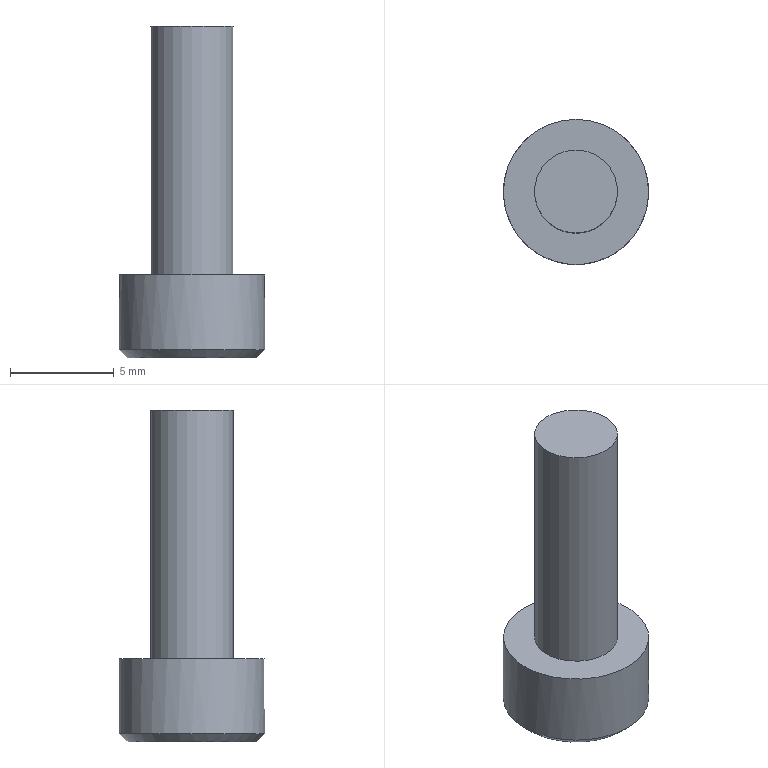Part | NX | features 5003_334_CB4-12 2 | 1 solid | 19 faces | box 7 x 7 x 16 mm | volume 285.33 mm3 | plane 15 | cylinder 2 | cone 2 | commonest cylinder face diameters 4 x1 7 x1
STEP:
#1=CARTESIAN_POINT('',(216.825,63.3,-140.18));
#2=VERTEX_POINT('',#1);
#3=CARTESIAN_POINT('',(216.825,66.4,-140.18));
#4=DIRECTION('',(0.,0.,1.));
#5=DIRECTION('',(0.,-1.,0.));
#6=AXIS2_PLACEMENT_3D('',#3,#4,#5);
#7=CIRCLE('',#6,3.1);
#8=EDGE_CURVE('',#2,#2,#7,.F.);
#9=ORIENTED_EDGE('',*,*,#8,.T.);
#10=EDGE_LOOP('',(#9));
#11=FACE_BOUND('',#10,.T.);
#12=CARTESIAN_POINT('',(215.093,66.4,-140.18));
#13=VERTEX_POINT('',#12);
#14=CARTESIAN_POINT('',(215.959,67.9,-140.18));
#15=VERTEX_POINT('',#14);
#16=CARTESIAN_POINT('',(215.093,66.4,-140.18));
#17=DIRECTION('',(0.5,0.866,0.));
#18=VECTOR('',#17,1000.);
#19=LINE('',#16,#18);
#20=EDGE_CURVE('',#13,#15,#19,.T.);
#21=ORIENTED_EDGE('',*,*,#20,.F.);
#22=CARTESIAN_POINT('',(215.959,64.9,-140.18));
#23=VERTEX_POINT('',#22);
#24=CARTESIAN_POINT('',(215.959,64.9,-140.18));
#25=DIRECTION('',(-0.5,0.866,0.));
#26=VECTOR('',#25,1000.);
#27=LINE('',#24,#26);
#28=EDGE_CURVE('',#23,#13,#27,.T.);
#29=ORIENTED_EDGE('',*,*,#28,.F.);
#30=CARTESIAN_POINT('',(217.691,64.9,-140.18));
#31=VERTEX_POINT('',#30);
#32=CARTESIAN_POINT('',(217.691,64.9,-140.18));
#33=DIRECTION('',(-1.,0.,0.));
#34=VECTOR('',#33,1000.);
#35=LINE('',#32,#34);
#36=EDGE_CURVE('',#31,#23,#35,.T.);
#37=ORIENTED_EDGE('',*,*,#36,.F.);
#38=CARTESIAN_POINT('',(218.557,66.4,-140.18));
#39=VERTEX_POINT('',#38);
#40=CARTESIAN_POINT('',(218.557,66.4,-140.18));
#41=DIRECTION('',(-0.5,-0.866,0.));
#42=VECTOR('',#41,1000.);
#43=LINE('',#40,#42);
#44=EDGE_CURVE('',#39,#31,#43,.T.);
#45=ORIENTED_EDGE('',*,*,#44,.F.);
#46=CARTESIAN_POINT('',(217.691,67.9,-140.18));
#47=VERTEX_POINT('',#46);
#48=CARTESIAN_POINT('',(217.691,67.9,-140.18));
#49=DIRECTION('',(0.5,-0.866,0.));
#50=VECTOR('',#49,1000.);
#51=LINE('',#48,#50);
#52=EDGE_CURVE('',#47,#39,#51,.T.);
#53=ORIENTED_EDGE('',*,*,#52,.F.);
#54=CARTESIAN_POINT('',(215.959,67.9,-140.18));
#55=DIRECTION('',(1.,0.,0.));
#56=VECTOR('',#55,1000.);
#57=LINE('',#54,#56);
#58=EDGE_CURVE('',#15,#47,#57,.T.);
#59=ORIENTED_EDGE('',*,*,#58,.F.);
#60=EDGE_LOOP('',(#21,#29,#37,#45,#53,#59));
#61=FACE_BOUND('',#60,.T.);
#62=CARTESIAN_POINT('',(220.325,66.4,-140.18));
#63=DIRECTION('',(0.,0.,1.));
#64=DIRECTION('',(0.,-1.,0.));
#65=AXIS2_PLACEMENT_3D('',#62,#63,#64);
#66=PLANE('',#65);
#67=ADVANCED_FACE('',(#11,#61),#66,.F.);
#68=CARTESIAN_POINT('',(216.825,68.4,-124.18));
#69=VERTEX_POINT('',#68);
#70=CARTESIAN_POINT('',(216.825,66.4,-124.18));
#71=DIRECTION('',(0.,0.,-1.));
#72=DIRECTION('',(0.,1.,0.));
#73=AXIS2_PLACEMENT_3D('',#70,#71,#72);
#74=CIRCLE('',#73,2.);
#75=EDGE_CURVE('',#69,#69,#74,.T.);
#76=ORIENTED_EDGE('',*,*,#75,.F.);
#77=EDGE_LOOP('',(#76));
#78=FACE_BOUND('',#77,.T.);
#79=CARTESIAN_POINT('',(216.825,66.4,-124.18));
#80=DIRECTION('',(0.,0.,-1.));
#81=DIRECTION('',(0.,1.,0.));
#82=AXIS2_PLACEMENT_3D('',#79,#80,#81);
#83=PLANE('',#82);
#84=ADVANCED_FACE('',(#78),#83,.F.);
#85=CARTESIAN_POINT('',(216.825,68.4,-136.18));
#86=VERTEX_POINT('',#85);
#87=CARTESIAN_POINT('',(216.825,66.4,-136.18));
#88=DIRECTION('',(0.,0.,-1.));
#89=DIRECTION('',(0.,1.,0.));
#90=AXIS2_PLACEMENT_3D('',#87,#88,#89);
#91=CIRCLE('',#90,2.);
#92=EDGE_CURVE('',#86,#86,#91,.T.);
#93=ORIENTED_EDGE('',*,*,#92,.F.);
#94=EDGE_LOOP('',(#93));
#95=FACE_BOUND('',#94,.T.);
#96=ORIENTED_EDGE('',*,*,#75,.T.);
#97=EDGE_LOOP('',(#96));
#98=FACE_BOUND('',#97,.T.);
#99=CARTESIAN_POINT('',(216.825,66.4,-140.18));
#100=DIRECTION('',(0.,0.,-1.));
#101=DIRECTION('',(0.,1.,0.));
#102=AXIS2_PLACEMENT_3D('',#99,#100,#101);
#103=CYLINDRICAL_SURFACE('',#102,2.);
#104=ADVANCED_FACE('',(#95,#98),#103,.T.);
#105=CARTESIAN_POINT('',(216.825,69.9,-136.18));
#106=VERTEX_POINT('',#105);
#107=CARTESIAN_POINT('',(216.825,66.4,-136.18));
#108=DIRECTION('',(0.,0.,-1.));
#109=DIRECTION('',(0.,1.,0.));
#110=AXIS2_PLACEMENT_3D('',#107,#108,#109);
#111=CIRCLE('',#110,3.5);
#112=EDGE_CURVE('',#106,#106,#111,.T.);
#113=ORIENTED_EDGE('',*,*,#112,.F.);
#114=EDGE_LOOP('',(#113));
#115=FACE_BOUND('',#114,.T.);
#116=ORIENTED_EDGE('',*,*,#92,.T.);
#117=EDGE_LOOP('',(#116));
#118=FACE_BOUND('',#117,.T.);
#119=CARTESIAN_POINT('',(218.825,66.4,-136.18));
#120=DIRECTION('',(0.,0.,-1.));
#121=DIRECTION('',(0.,1.,0.));
#122=AXIS2_PLACEMENT_3D('',#119,#120,#121);
#123=PLANE('',#122);
#124=ADVANCED_FACE('',(#115,#118),#123,.F.);
#125=CARTESIAN_POINT('',(216.825,62.9,-139.78));
#126=VERTEX_POINT('',#125);
#127=CARTESIAN_POINT('',(216.825,66.4,-139.78));
#128=DIRECTION('',(0.,0.,1.));
#129=DIRECTION('',(0.,-1.,0.));
#130=AXIS2_PLACEMENT_3D('',#127,#128,#129);
#131=CIRCLE('',#130,3.5);
#132=EDGE_CURVE('',#126,#126,#131,.T.);
#133=ORIENTED_EDGE('',*,*,#132,.T.);
#134=EDGE_LOOP('',(#133));
#135=FACE_BOUND('',#134,.T.);
#136=ORIENTED_EDGE('',*,*,#112,.T.);
#137=EDGE_LOOP('',(#136));
#138=FACE_BOUND('',#137,.T.);
#139=CARTESIAN_POINT('',(216.825,66.4,-140.18));
#140=DIRECTION('',(0.,0.,-1.));
#141=DIRECTION('',(0.,1.,0.));
#142=AXIS2_PLACEMENT_3D('',#139,#140,#141);
#143=CYLINDRICAL_SURFACE('',#142,3.5);
#144=ADVANCED_FACE('',(#135,#138),#143,.T.);
#145=ORIENTED_EDGE('',*,*,#132,.F.);
#146=EDGE_LOOP('',(#145));
#147=FACE_BOUND('',#146,.T.);
#148=ORIENTED_EDGE('',*,*,#8,.F.);
#149=EDGE_LOOP('',(#148));
#150=FACE_BOUND('',#149,.T.);
#151=CARTESIAN_POINT('',(216.825,66.4,-140.18));
#152=DIRECTION('',(0.,0.,1.));
#153=DIRECTION('',(0.,-1.,0.));
#154=AXIS2_PLACEMENT_3D('',#151,#152,#153);
#155=CONICAL_SURFACE('',#154,3.1,0.7854);
#156=ADVANCED_FACE('',(#147,#150),#155,.T.);
#157=CARTESIAN_POINT('',(215.959,64.9,-138.18));
#158=VERTEX_POINT('',#157);
#159=CARTESIAN_POINT('',(215.526,65.65,-138.18));
#160=VERTEX_POINT('',#159);
#161=CARTESIAN_POINT('',(215.959,64.9,-138.18));
#162=DIRECTION('',(-0.5,0.866,0.));
#163=VECTOR('',#162,1000.);
#164=LINE('',#161,#163);
#165=EDGE_CURVE('',#158,#160,#164,.T.);
#166=ORIENTED_EDGE('',*,*,#165,.F.);
#167=CARTESIAN_POINT('',(215.959,64.9,-138.18));
#168=DIRECTION('',(0.,0.,-1.));
#169=VECTOR('',#168,1000.);
#170=LINE('',#167,#169);
#171=EDGE_CURVE('',#158,#23,#170,.T.);
#172=ORIENTED_EDGE('',*,*,#171,.T.);
#173=ORIENTED_EDGE('',*,*,#28,.T.);
#174=CARTESIAN_POINT('',(215.093,66.4,-138.18));
#175=VERTEX_POINT('',#174);
#176=CARTESIAN_POINT('',(215.093,66.4,-138.18));
#177=DIRECTION('',(0.,0.,-1.));
#178=VECTOR('',#177,1000.);
#179=LINE('',#176,#178);
#180=EDGE_CURVE('',#175,#13,#179,.T.);
#181=ORIENTED_EDGE('',*,*,#180,.F.);
#182=CARTESIAN_POINT('',(215.959,64.9,-138.18));
#183=DIRECTION('',(-0.5,0.866,0.));
#184=VECTOR('',#183,1000.);
#185=LINE('',#182,#184);
#186=EDGE_CURVE('',#160,#175,#185,.T.);
#187=ORIENTED_EDGE('',*,*,#186,.F.);
#188=EDGE_LOOP('',(#166,#172,#173,#181,#187));
#189=FACE_BOUND('',#188,.T.);
#190=CARTESIAN_POINT('',(215.959,64.9,-138.18));
#191=DIRECTION('',(-0.866,-0.5,0.));
#192=DIRECTION('',(0.5,-0.866,0.));
#193=AXIS2_PLACEMENT_3D('',#190,#191,#192);
#194=PLANE('',#193);
#195=ADVANCED_FACE('',(#189),#194,.F.);
#196=CARTESIAN_POINT('',(217.691,64.9,-138.18));
#197=VERTEX_POINT('',#196);
#198=CARTESIAN_POINT('',(216.825,64.9,-138.18));
#199=VERTEX_POINT('',#198);
#200=CARTESIAN_POINT('',(217.691,64.9,-138.18));
#201=DIRECTION('',(-1.,0.,0.));
#202=VECTOR('',#201,1000.);
#203=LINE('',#200,#202);
#204=EDGE_CURVE('',#197,#199,#203,.T.);
#205=ORIENTED_EDGE('',*,*,#204,.F.);
#206=CARTESIAN_POINT('',(217.691,64.9,-138.18));
#207=DIRECTION('',(0.,0.,-1.));
#208=VECTOR('',#207,1000.);
#209=LINE('',#206,#208);
#210=EDGE_CURVE('',#197,#31,#209,.T.);
#211=ORIENTED_EDGE('',*,*,#210,.T.);
#212=ORIENTED_EDGE('',*,*,#36,.T.);
#213=ORIENTED_EDGE('',*,*,#171,.F.);
#214=CARTESIAN_POINT('',(217.691,64.9,-138.18));
#215=DIRECTION('',(-1.,0.,0.));
#216=VECTOR('',#215,1000.);
#217=LINE('',#214,#216);
#218=EDGE_CURVE('',#199,#158,#217,.T.);
#219=ORIENTED_EDGE('',*,*,#218,.F.);
#220=EDGE_LOOP('',(#205,#211,#212,#213,#219));
#221=FACE_BOUND('',#220,.T.);
#222=CARTESIAN_POINT('',(217.691,64.9,-138.18));
#223=DIRECTION('',(0.,-1.,0.));
#224=DIRECTION('',(0.,0.,-1.));
#225=AXIS2_PLACEMENT_3D('',#222,#223,#224);
#226=PLANE('',#225);
#227=ADVANCED_FACE('',(#221),#226,.F.);
#228=CARTESIAN_POINT('',(218.557,66.4,-138.18));
#229=VERTEX_POINT('',#228);
#230=CARTESIAN_POINT('',(218.124,65.65,-138.18));
#231=VERTEX_POINT('',#230);
#232=CARTESIAN_POINT('',(218.557,66.4,-138.18));
#233=DIRECTION('',(-0.5,-0.866,0.));
#234=VECTOR('',#233,1000.);
#235=LINE('',#232,#234);
#236=EDGE_CURVE('',#229,#231,#235,.T.);
#237=ORIENTED_EDGE('',*,*,#236,.F.);
#238=CARTESIAN_POINT('',(218.557,66.4,-138.18));
#239=DIRECTION('',(0.,0.,-1.));
#240=VECTOR('',#239,1000.);
#241=LINE('',#238,#240);
#242=EDGE_CURVE('',#229,#39,#241,.T.);
#243=ORIENTED_EDGE('',*,*,#242,.T.);
#244=ORIENTED_EDGE('',*,*,#44,.T.);
#245=ORIENTED_EDGE('',*,*,#210,.F.);
#246=CARTESIAN_POINT('',(218.557,66.4,-138.18));
#247=DIRECTION('',(-0.5,-0.866,0.));
#248=VECTOR('',#247,1000.);
#249=LINE('',#246,#248);
#250=EDGE_CURVE('',#231,#197,#249,.T.);
#251=ORIENTED_EDGE('',*,*,#250,.F.);
#252=EDGE_LOOP('',(#237,#243,#244,#245,#251));
#253=FACE_BOUND('',#252,.T.);
#254=CARTESIAN_POINT('',(218.557,66.4,-138.18));
#255=DIRECTION('',(0.866,-0.5,0.));
#256=DIRECTION('',(0.5,0.866,0.));
#257=AXIS2_PLACEMENT_3D('',#254,#255,#256);
#258=PLANE('',#257);
#259=ADVANCED_FACE('',(#253),#258,.F.);
#260=CARTESIAN_POINT('',(217.691,67.9,-138.18));
#261=VERTEX_POINT('',#260);
#262=CARTESIAN_POINT('',(218.124,67.15,-138.18));
#263=VERTEX_POINT('',#262);
#264=CARTESIAN_POINT('',(217.691,67.9,-138.18));
#265=DIRECTION('',(0.5,-0.866,0.));
#266=VECTOR('',#265,1000.);
#267=LINE('',#264,#266);
#268=EDGE_CURVE('',#261,#263,#267,.T.);
#269=ORIENTED_EDGE('',*,*,#268,.F.);
#270=CARTESIAN_POINT('',(217.691,67.9,-138.18));
#271=DIRECTION('',(0.,0.,-1.));
#272=VECTOR('',#271,1000.);
#273=LINE('',#270,#272);
#274=EDGE_CURVE('',#261,#47,#273,.T.);
#275=ORIENTED_EDGE('',*,*,#274,.T.);
#276=ORIENTED_EDGE('',*,*,#52,.T.);
#277=ORIENTED_EDGE('',*,*,#242,.F.);
#278=CARTESIAN_POINT('',(217.691,67.9,-138.18));
#279=DIRECTION('',(0.5,-0.866,0.));
#280=VECTOR('',#279,1000.);
#281=LINE('',#278,#280);
#282=EDGE_CURVE('',#263,#229,#281,.T.);
#283=ORIENTED_EDGE('',*,*,#282,.F.);
#284=EDGE_LOOP('',(#269,#275,#276,#277,#283));
#285=FACE_BOUND('',#284,.T.);
#286=CARTESIAN_POINT('',(217.691,67.9,-138.18));
#287=DIRECTION('',(0.866,0.5,0.));
#288=DIRECTION('',(-0.5,0.866,0.));
#289=AXIS2_PLACEMENT_3D('',#286,#287,#288);
#290=PLANE('',#289);
#291=ADVANCED_FACE('',(#285),#290,.F.);
#292=CARTESIAN_POINT('',(215.959,67.9,-138.18));
#293=VERTEX_POINT('',#292);
#294=CARTESIAN_POINT('',(216.825,67.9,-138.18));
#295=VERTEX_POINT('',#294);
#296=CARTESIAN_POINT('',(215.959,67.9,-138.18));
#297=DIRECTION('',(1.,0.,0.));
#298=VECTOR('',#297,1000.);
#299=LINE('',#296,#298);
#300=EDGE_CURVE('',#293,#295,#299,.T.);
#301=ORIENTED_EDGE('',*,*,#300,.F.);
#302=CARTESIAN_POINT('',(215.959,67.9,-138.18));
#303=DIRECTION('',(0.,0.,-1.));
#304=VECTOR('',#303,1000.);
#305=LINE('',#302,#304);
#306=EDGE_CURVE('',#293,#15,#305,.T.);
#307=ORIENTED_EDGE('',*,*,#306,.T.);
#308=ORIENTED_EDGE('',*,*,#58,.T.);
#309=ORIENTED_EDGE('',*,*,#274,.F.);
#310=CARTESIAN_POINT('',(215.959,67.9,-138.18));
#311=DIRECTION('',(1.,0.,0.));
#312=VECTOR('',#311,1000.);
#313=LINE('',#310,#312);
#314=EDGE_CURVE('',#295,#261,#313,.T.);
#315=ORIENTED_EDGE('',*,*,#314,.F.);
#316=EDGE_LOOP('',(#301,#307,#308,#309,#315));
#317=FACE_BOUND('',#316,.T.);
#318=CARTESIAN_POINT('',(215.959,67.9,-138.18));
#319=DIRECTION('',(0.,1.,0.));
#320=DIRECTION('',(0.,0.,1.));
#321=AXIS2_PLACEMENT_3D('',#318,#319,#320);
#322=PLANE('',#321);
#323=ADVANCED_FACE('',(#317),#322,.F.);
#324=CARTESIAN_POINT('',(215.526,67.15,-138.18));
#325=VERTEX_POINT('',#324);
#326=CARTESIAN_POINT('',(215.093,66.4,-138.18));
#327=DIRECTION('',(0.5,0.866,0.));
#328=VECTOR('',#327,1000.);
#329=LINE('',#326,#328);
#330=EDGE_CURVE('',#175,#325,#329,.T.);
#331=ORIENTED_EDGE('',*,*,#330,.F.);
#332=ORIENTED_EDGE('',*,*,#180,.T.);
#333=ORIENTED_EDGE('',*,*,#20,.T.);
#334=ORIENTED_EDGE('',*,*,#306,.F.);
#335=CARTESIAN_POINT('',(215.093,66.4,-138.18));
#336=DIRECTION('',(0.5,0.866,0.));
#337=VECTOR('',#336,1000.);
#338=LINE('',#335,#337);
#339=EDGE_CURVE('',#325,#293,#338,.T.);
#340=ORIENTED_EDGE('',*,*,#339,.F.);
#341=EDGE_LOOP('',(#331,#332,#333,#334,#340));
#342=FACE_BOUND('',#341,.T.);
#343=CARTESIAN_POINT('',(215.093,66.4,-138.18));
#344=DIRECTION('',(-0.866,0.5,0.));
#345=DIRECTION('',(-0.5,-0.866,0.));
#346=AXIS2_PLACEMENT_3D('',#343,#344,#345);
#347=PLANE('',#346);
#348=ADVANCED_FACE('',(#342),#347,.F.);
#349=ORIENTED_EDGE('',*,*,#314,.T.);
#350=ORIENTED_EDGE('',*,*,#268,.T.);
#351=CARTESIAN_POINT('',(216.825,66.4,-138.18));
#352=DIRECTION('',(0.,0.,-1.));
#353=DIRECTION('',(-1.,0.,0.));
#354=AXIS2_PLACEMENT_3D('',#351,#352,#353);
#355=CIRCLE('',#354,1.5);
#356=EDGE_CURVE('',#295,#263,#355,.T.);
#357=ORIENTED_EDGE('',*,*,#356,.F.);
#358=EDGE_LOOP('',(#349,#350,#357));
#359=FACE_BOUND('',#358,.T.);
#360=CARTESIAN_POINT('',(216.825,66.4,-138.18));
#361=DIRECTION('',(0.,0.,-1.));
#362=DIRECTION('',(0.,1.,0.));
#363=AXIS2_PLACEMENT_3D('',#360,#361,#362);
#364=PLANE('',#363);
#365=ADVANCED_FACE('',(#359),#364,.T.);
#366=ORIENTED_EDGE('',*,*,#282,.T.);
#367=ORIENTED_EDGE('',*,*,#236,.T.);
#368=CARTESIAN_POINT('',(216.825,66.4,-138.18));
#369=DIRECTION('',(0.,0.,-1.));
#370=DIRECTION('',(-1.,0.,0.));
#371=AXIS2_PLACEMENT_3D('',#368,#369,#370);
#372=CIRCLE('',#371,1.5);
#373=EDGE_CURVE('',#263,#231,#372,.T.);
#374=ORIENTED_EDGE('',*,*,#373,.F.);
#375=EDGE_LOOP('',(#366,#367,#374));
#376=FACE_BOUND('',#375,.T.);
#377=CARTESIAN_POINT('',(216.825,66.4,-138.18));
#378=DIRECTION('',(0.,0.,-1.));
#379=DIRECTION('',(0.,1.,0.));
#380=AXIS2_PLACEMENT_3D('',#377,#378,#379);
#381=PLANE('',#380);
#382=ADVANCED_FACE('',(#376),#381,.T.);
#383=ORIENTED_EDGE('',*,*,#250,.T.);
#384=ORIENTED_EDGE('',*,*,#204,.T.);
#385=CARTESIAN_POINT('',(216.825,66.4,-138.18));
#386=DIRECTION('',(0.,0.,-1.));
#387=DIRECTION('',(-1.,0.,0.));
#388=AXIS2_PLACEMENT_3D('',#385,#386,#387);
#389=CIRCLE('',#388,1.5);
#390=EDGE_CURVE('',#231,#199,#389,.T.);
#391=ORIENTED_EDGE('',*,*,#390,.F.);
#392=EDGE_LOOP('',(#383,#384,#391));
#393=FACE_BOUND('',#392,.T.);
#394=CARTESIAN_POINT('',(216.825,66.4,-138.18));
#395=DIRECTION('',(0.,0.,-1.));
#396=DIRECTION('',(0.,1.,0.));
#397=AXIS2_PLACEMENT_3D('',#394,#395,#396);
#398=PLANE('',#397);
#399=ADVANCED_FACE('',(#393),#398,.T.);
#400=ORIENTED_EDGE('',*,*,#218,.T.);
#401=ORIENTED_EDGE('',*,*,#165,.T.);
#402=CARTESIAN_POINT('',(216.825,66.4,-138.18));
#403=DIRECTION('',(0.,0.,-1.));
#404=DIRECTION('',(-1.,0.,0.));
#405=AXIS2_PLACEMENT_3D('',#402,#403,#404);
#406=CIRCLE('',#405,1.5);
#407=EDGE_CURVE('',#199,#160,#406,.T.);
#408=ORIENTED_EDGE('',*,*,#407,.F.);
#409=EDGE_LOOP('',(#400,#401,#408));
#410=FACE_BOUND('',#409,.T.);
#411=CARTESIAN_POINT('',(216.825,66.4,-138.18));
#412=DIRECTION('',(0.,0.,-1.));
#413=DIRECTION('',(0.,1.,0.));
#414=AXIS2_PLACEMENT_3D('',#411,#412,#413);
#415=PLANE('',#414);
#416=ADVANCED_FACE('',(#410),#415,.T.);
#417=ORIENTED_EDGE('',*,*,#186,.T.);
#418=ORIENTED_EDGE('',*,*,#330,.T.);
#419=CARTESIAN_POINT('',(216.825,66.4,-138.18));
#420=DIRECTION('',(0.,0.,-1.));
#421=DIRECTION('',(-1.,0.,0.));
#422=AXIS2_PLACEMENT_3D('',#419,#420,#421);
#423=CIRCLE('',#422,1.5);
#424=EDGE_CURVE('',#160,#325,#423,.T.);
#425=ORIENTED_EDGE('',*,*,#424,.F.);
#426=EDGE_LOOP('',(#417,#418,#425));
#427=FACE_BOUND('',#426,.T.);
#428=CARTESIAN_POINT('',(216.825,66.4,-138.18));
#429=DIRECTION('',(0.,0.,-1.));
#430=DIRECTION('',(0.,1.,0.));
#431=AXIS2_PLACEMENT_3D('',#428,#429,#430);
#432=PLANE('',#431);
#433=ADVANCED_FACE('',(#427),#432,.T.);
#434=ORIENTED_EDGE('',*,*,#339,.T.);
#435=ORIENTED_EDGE('',*,*,#300,.T.);
#436=CARTESIAN_POINT('',(216.825,66.4,-138.18));
#437=DIRECTION('',(0.,0.,-1.));
#438=DIRECTION('',(-1.,0.,0.));
#439=AXIS2_PLACEMENT_3D('',#436,#437,#438);
#440=CIRCLE('',#439,1.5);
#441=EDGE_CURVE('',#325,#295,#440,.T.);
#442=ORIENTED_EDGE('',*,*,#441,.F.);
#443=EDGE_LOOP('',(#434,#435,#442));
#444=FACE_BOUND('',#443,.T.);
#445=CARTESIAN_POINT('',(216.825,66.4,-138.18));
#446=DIRECTION('',(0.,0.,-1.));
#447=DIRECTION('',(0.,1.,0.));
#448=AXIS2_PLACEMENT_3D('',#445,#446,#447);
#449=PLANE('',#448);
#450=ADVANCED_FACE('',(#444),#449,.T.);
#451=ORIENTED_EDGE('',*,*,#441,.T.);
#452=ORIENTED_EDGE('',*,*,#356,.T.);
#453=ORIENTED_EDGE('',*,*,#373,.T.);
#454=ORIENTED_EDGE('',*,*,#390,.T.);
#455=ORIENTED_EDGE('',*,*,#407,.T.);
#456=ORIENTED_EDGE('',*,*,#424,.T.);
#457=EDGE_LOOP('',(#451,#452,#453,#454,#455,#456));
#458=FACE_BOUND('',#457,.T.);
#459=CARTESIAN_POINT('',(216.825,66.4,-137.279));
#460=VERTEX_POINT('',#459);
#461=VERTEX_LOOP('',#460);
#462=FACE_BOUND('',#461,.T.);
#463=CARTESIAN_POINT('',(216.825,66.4,-137.279));
#464=DIRECTION('',(0.,0.,-1.));
#465=DIRECTION('',(-1.,0.,0.));
#466=AXIS2_PLACEMENT_3D('',#463,#464,#465);
#467=CONICAL_SURFACE('',#466,0.,1.03);
#468=ADVANCED_FACE('',(#458,#462),#467,.F.);
#469=CLOSED_SHELL('',(#67,#84,#104,#124,#144,#156,#195,#227,#259,#291,#323,#348,#365,#382,#399,#416,#433,#450,#468));
#470=MANIFOLD_SOLID_BREP('',#469);
#471=(LENGTH_UNIT()NAMED_UNIT(*)SI_UNIT(.MILLI.,.METRE.));
#472=UNCERTAINTY_MEASURE_WITH_UNIT(LENGTH_MEASURE(0.00001),#471,'','');
#473=(NAMED_UNIT(*)PLANE_ANGLE_UNIT()SI_UNIT($,.RADIAN.));
#474=(NAMED_UNIT(*)SI_UNIT($,.STERADIAN.)SOLID_ANGLE_UNIT());
#475=(GEOMETRIC_REPRESENTATION_CONTEXT(3)GLOBAL_UNCERTAINTY_ASSIGNED_CONTEXT((#472))GLOBAL_UNIT_ASSIGNED_CONTEXT((#471,#473,#474))REPRESENTATION_CONTEXT('',''));
#476=ADVANCED_BREP_SHAPE_REPRESENTATION('',(#470),#475);